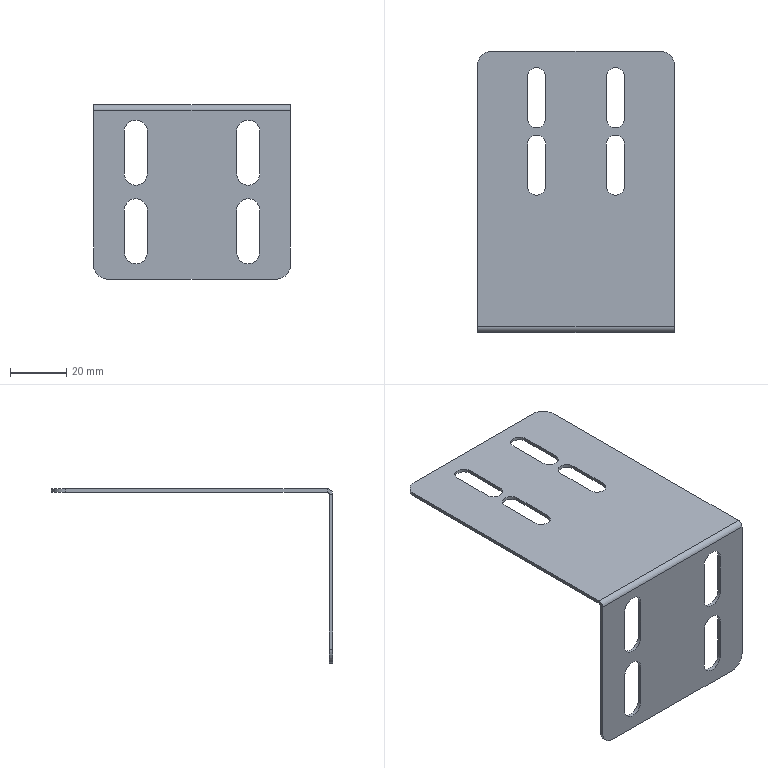Part | 1 solid | 54 faces | box 70 x 100 x 62 mm | volume 11974 mm3 | plane 28 | cylinder 26 | commonest cylinder face diameters 8.2 x12 6.4 x8 10 x4 1.48 x1 3.88 x1